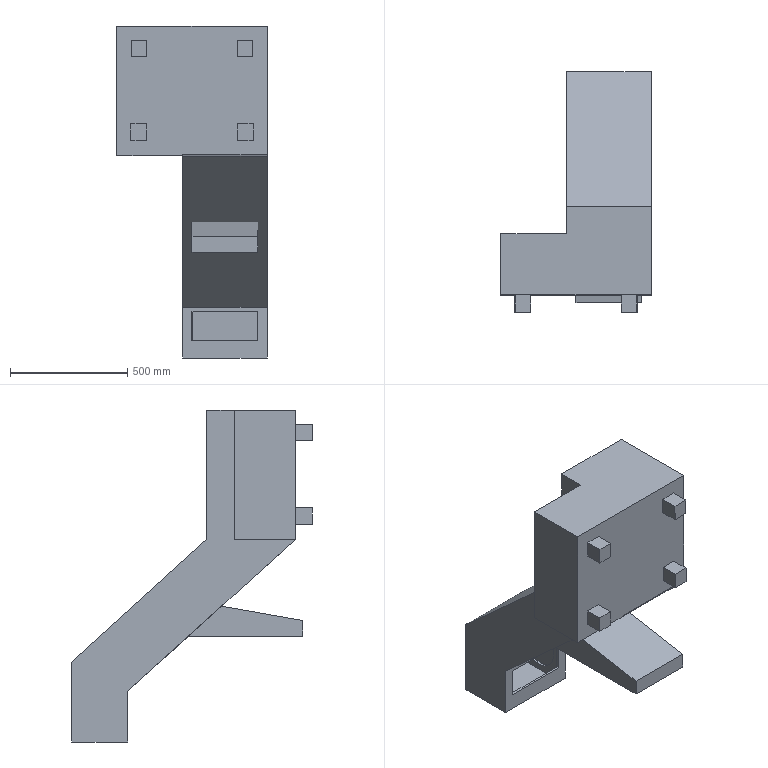Part | STEP file | Boss-Extrude 8 | 1 solid | 97 faces | box 640 x 1025 x 1413 mm | volume 96392257 mm3 | plane 73 | cylinder 24 | commonest cylinder face diameters 44 x4 180 x4 324 x4 18.203 x2 23.777 x2 24.528 x2